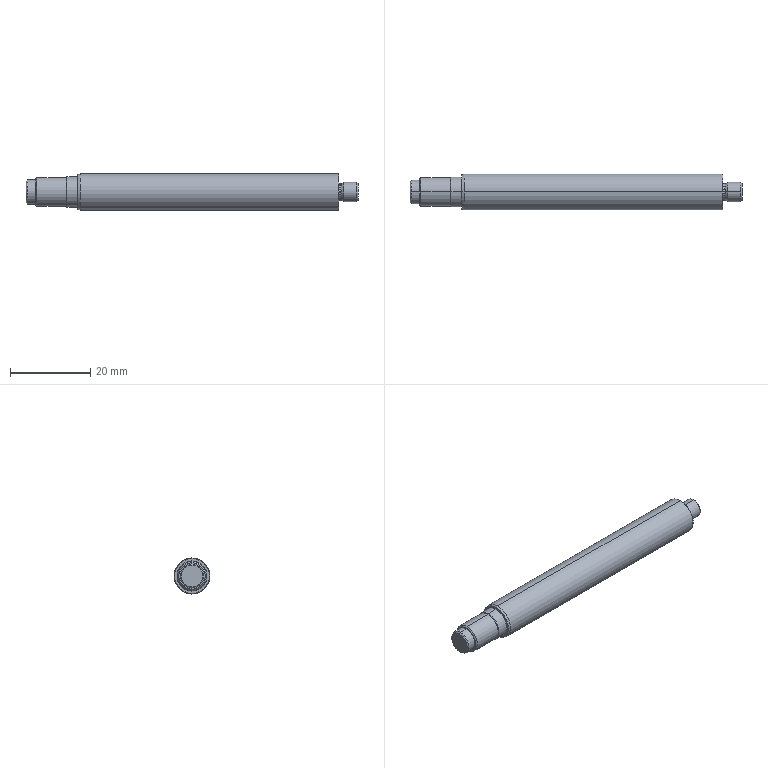Part | STEP file | 2026.6.15-Main Assembly图.sldasm-Part-245 | 1 solid | 35 faces | box 82.8 x 9 x 9 mm | volume 4725 mm3 | cone 12 | cylinder 12 | torus 6 | plane 5 | commonest cylinder face diameters 4.11 x2 4.8 x2 6 x2 7.2 x2 7.5 x2 9 x2
STEP:
#1=CARTESIAN_POINT('',(-1606.188,1424.264,3405.386));
#2=VERTEX_POINT('',#1);
#3=CARTESIAN_POINT('',(-1606.188,1424.264,3410.786));
#4=VERTEX_POINT('',#3);
#5=CARTESIAN_POINT('',(-1606.188,1424.264,3408.086));
#6=DIRECTION('',(1.,0.,0.));
#7=DIRECTION('',(0.,0.,-1.));
#8=AXIS2_PLACEMENT_3D('',#5,#6,#7);
#9=CIRCLE('',#8,2.7);
#10=EDGE_CURVE('',#2,#4,#9,.T.);
#11=ORIENTED_EDGE('',*,*,#10,.F.);
#12=CARTESIAN_POINT('',(-1606.188,1424.264,3408.086));
#13=DIRECTION('',(1.,0.,0.));
#14=DIRECTION('',(0.,0.,-1.));
#15=AXIS2_PLACEMENT_3D('',#12,#13,#14);
#16=CIRCLE('',#15,2.7);
#17=EDGE_CURVE('',#4,#2,#16,.T.);
#18=ORIENTED_EDGE('',*,*,#17,.F.);
#19=EDGE_LOOP('',(#11,#18));
#20=FACE_OUTER_BOUND('',#19,.T.);
#21=CARTESIAN_POINT('',(-1606.188,1424.264,3408.086));
#22=DIRECTION('',(-1.,0.,0.));
#23=DIRECTION('',(0.,0.,1.));
#24=AXIS2_PLACEMENT_3D('',#21,#22,#23);
#25=PLANE('',#24);
#26=ADVANCED_FACE('',(#20),#25,.T.);
#27=CARTESIAN_POINT('',(-1605.888,1424.264,3411.086));
#28=VERTEX_POINT('',#27);
#29=CARTESIAN_POINT('',(-1605.888,1424.264,3411.086));
#30=DIRECTION('',(0.7071,0.,0.7071));
#31=VECTOR('',#30,1000.);
#32=LINE('',#29,#31);
#33=EDGE_CURVE('',#4,#28,#32,.T.);
#34=ORIENTED_EDGE('',*,*,#33,.F.);
#35=ORIENTED_EDGE('',*,*,#17,.T.);
#36=CARTESIAN_POINT('',(-1605.888,1424.264,3405.086));
#37=VERTEX_POINT('',#36);
#38=CARTESIAN_POINT('',(-1605.888,1424.264,3405.086));
#39=DIRECTION('',(0.7071,0.,-0.7071));
#40=VECTOR('',#39,1000.);
#41=LINE('',#38,#40);
#42=EDGE_CURVE('',#2,#37,#41,.T.);
#43=ORIENTED_EDGE('',*,*,#42,.T.);
#44=CARTESIAN_POINT('',(-1605.888,1424.264,3408.086));
#45=DIRECTION('',(1.,0.,0.));
#46=DIRECTION('',(0.,0.,-1.));
#47=AXIS2_PLACEMENT_3D('',#44,#45,#46);
#48=CIRCLE('',#47,3.);
#49=EDGE_CURVE('',#28,#37,#48,.T.);
#50=ORIENTED_EDGE('',*,*,#49,.F.);
#51=EDGE_LOOP('',(#34,#35,#43,#50));
#52=FACE_OUTER_BOUND('',#51,.T.);
#53=CARTESIAN_POINT('',(-1605.888,1424.264,3408.086));
#54=DIRECTION('',(1.,0.,0.));
#55=DIRECTION('',(0.,0.,1.));
#56=AXIS2_PLACEMENT_3D('',#53,#54,#55);
#57=CONICAL_SURFACE('',#56,3.,0.7854);
#58=ADVANCED_FACE('',(#52),#57,.T.);
#59=CARTESIAN_POINT('',(-1523.388,1424.264,3410.186));
#60=VERTEX_POINT('',#59);
#61=CARTESIAN_POINT('',(-1523.388,1424.264,3405.986));
#62=VERTEX_POINT('',#61);
#63=CARTESIAN_POINT('',(-1523.388,1424.264,3408.086));
#64=DIRECTION('',(-1.,0.,0.));
#65=DIRECTION('',(0.,0.,1.));
#66=AXIS2_PLACEMENT_3D('',#63,#64,#65);
#67=CIRCLE('',#66,2.1);
#68=EDGE_CURVE('',#60,#62,#67,.T.);
#69=ORIENTED_EDGE('',*,*,#68,.F.);
#70=CARTESIAN_POINT('',(-1523.388,1424.264,3408.086));
#71=DIRECTION('',(-1.,0.,0.));
#72=DIRECTION('',(0.,0.,1.));
#73=AXIS2_PLACEMENT_3D('',#70,#71,#72);
#74=CIRCLE('',#73,2.1);
#75=EDGE_CURVE('',#62,#60,#74,.T.);
#76=ORIENTED_EDGE('',*,*,#75,.F.);
#77=EDGE_LOOP('',(#69,#76));
#78=FACE_OUTER_BOUND('',#77,.T.);
#79=CARTESIAN_POINT('',(-1523.388,1424.264,3408.086));
#80=DIRECTION('',(-1.,0.,0.));
#81=DIRECTION('',(0.,0.,1.));
#82=AXIS2_PLACEMENT_3D('',#79,#80,#81);
#83=PLANE('',#82);
#84=ADVANCED_FACE('',(#78),#83,.F.);
#85=CARTESIAN_POINT('',(-1603.788,1424.264,3411.086));
#86=VERTEX_POINT('',#85);
#87=CARTESIAN_POINT('',(-1603.788,1424.264,3411.086));
#88=DIRECTION('',(1.,0.,0.));
#89=VECTOR('',#88,1000.);
#90=LINE('',#87,#89);
#91=EDGE_CURVE('',#28,#86,#90,.T.);
#92=ORIENTED_EDGE('',*,*,#91,.F.);
#93=ORIENTED_EDGE('',*,*,#49,.T.);
#94=CARTESIAN_POINT('',(-1603.788,1424.264,3405.086));
#95=VERTEX_POINT('',#94);
#96=CARTESIAN_POINT('',(-1603.788,1424.264,3405.086));
#97=DIRECTION('',(1.,0.,0.));
#98=VECTOR('',#97,1000.);
#99=LINE('',#96,#98);
#100=EDGE_CURVE('',#37,#95,#99,.T.);
#101=ORIENTED_EDGE('',*,*,#100,.T.);
#102=CARTESIAN_POINT('',(-1603.788,1424.264,3408.086));
#103=DIRECTION('',(1.,0.,0.));
#104=DIRECTION('',(0.,0.,-1.));
#105=AXIS2_PLACEMENT_3D('',#102,#103,#104);
#106=CIRCLE('',#105,3.);
#107=EDGE_CURVE('',#86,#95,#106,.T.);
#108=ORIENTED_EDGE('',*,*,#107,.F.);
#109=EDGE_LOOP('',(#92,#93,#101,#108));
#110=FACE_OUTER_BOUND('',#109,.T.);
#111=CARTESIAN_POINT('',(-1603.788,1424.264,3408.086));
#112=DIRECTION('',(1.,0.,0.));
#113=DIRECTION('',(0.,0.,1.));
#114=AXIS2_PLACEMENT_3D('',#111,#112,#113);
#115=CYLINDRICAL_SURFACE('',#114,3.);
#116=ADVANCED_FACE('',(#110),#115,.T.);
#117=CARTESIAN_POINT('',(-1523.688,1424.264,3405.686));
#118=VERTEX_POINT('',#117);
#119=CARTESIAN_POINT('',(-1523.688,1424.264,3405.686));
#120=DIRECTION('',(0.7071,0.,0.7071));
#121=VECTOR('',#120,1000.);
#122=LINE('',#119,#121);
#123=EDGE_CURVE('',#118,#62,#122,.T.);
#124=ORIENTED_EDGE('',*,*,#123,.T.);
#125=ORIENTED_EDGE('',*,*,#75,.T.);
#126=CARTESIAN_POINT('',(-1523.688,1424.264,3410.486));
#127=VERTEX_POINT('',#126);
#128=CARTESIAN_POINT('',(-1523.688,1424.264,3410.486));
#129=DIRECTION('',(0.7071,0.,-0.7071));
#130=VECTOR('',#129,1000.);
#131=LINE('',#128,#130);
#132=EDGE_CURVE('',#127,#60,#131,.T.);
#133=ORIENTED_EDGE('',*,*,#132,.F.);
#134=CARTESIAN_POINT('',(-1523.688,1424.264,3408.086));
#135=DIRECTION('',(-1.,0.,0.));
#136=DIRECTION('',(0.,0.,1.));
#137=AXIS2_PLACEMENT_3D('',#134,#135,#136);
#138=CIRCLE('',#137,2.4);
#139=EDGE_CURVE('',#118,#127,#138,.T.);
#140=ORIENTED_EDGE('',*,*,#139,.F.);
#141=EDGE_LOOP('',(#124,#125,#133,#140));
#142=FACE_OUTER_BOUND('',#141,.T.);
#143=CARTESIAN_POINT('',(-1523.688,1424.264,3408.086));
#144=DIRECTION('',(-1.,0.,0.));
#145=DIRECTION('',(0.,0.,-1.));
#146=AXIS2_PLACEMENT_3D('',#143,#144,#145);
#147=CONICAL_SURFACE('',#146,2.4,0.7854);
#148=ADVANCED_FACE('',(#142),#147,.T.);
#149=CARTESIAN_POINT('',(-1603.788,1424.264,3404.786));
#150=VERTEX_POINT('',#149);
#151=CARTESIAN_POINT('',(-1603.788,1424.264,3411.386));
#152=VERTEX_POINT('',#151);
#153=CARTESIAN_POINT('',(-1603.788,1424.264,3408.086));
#154=DIRECTION('',(1.,0.,0.));
#155=DIRECTION('',(0.,0.,-1.));
#156=AXIS2_PLACEMENT_3D('',#153,#154,#155);
#157=CIRCLE('',#156,3.3);
#158=EDGE_CURVE('',#150,#152,#157,.T.);
#159=ORIENTED_EDGE('',*,*,#158,.F.);
#160=CARTESIAN_POINT('',(-1603.788,1424.264,3408.086));
#161=DIRECTION('',(1.,0.,0.));
#162=DIRECTION('',(0.,0.,-1.));
#163=AXIS2_PLACEMENT_3D('',#160,#161,#162);
#164=CIRCLE('',#163,3.3);
#165=EDGE_CURVE('',#152,#150,#164,.T.);
#166=ORIENTED_EDGE('',*,*,#165,.F.);
#167=EDGE_LOOP('',(#159,#166));
#168=FACE_OUTER_BOUND('',#167,.T.);
#169=CARTESIAN_POINT('',(-1603.788,1424.264,3408.086));
#170=DIRECTION('',(1.,0.,0.));
#171=DIRECTION('',(0.,0.,-1.));
#172=AXIS2_PLACEMENT_3D('',#169,#170,#171);
#173=CIRCLE('',#172,3.);
#174=EDGE_CURVE('',#95,#86,#173,.T.);
#175=ORIENTED_EDGE('',*,*,#174,.T.);
#176=ORIENTED_EDGE('',*,*,#107,.T.);
#177=EDGE_LOOP('',(#175,#176));
#178=FACE_BOUND('',#177,.T.);
#179=CARTESIAN_POINT('',(-1603.788,1425.764,3408.086));
#180=DIRECTION('',(-1.,0.,0.));
#181=DIRECTION('',(0.,0.,1.));
#182=AXIS2_PLACEMENT_3D('',#179,#180,#181);
#183=PLANE('',#182);
#184=ADVANCED_FACE('',(#168,#178),#183,.T.);
#185=CARTESIAN_POINT('',(-1526.988,1424.264,3405.686));
#186=VERTEX_POINT('',#185);
#187=CARTESIAN_POINT('',(-1528.188,1424.264,3405.686));
#188=DIRECTION('',(1.,0.,0.));
#189=VECTOR('',#188,1000.);
#190=LINE('',#187,#189);
#191=EDGE_CURVE('',#186,#118,#190,.T.);
#192=ORIENTED_EDGE('',*,*,#191,.T.);
#193=ORIENTED_EDGE('',*,*,#139,.T.);
#194=CARTESIAN_POINT('',(-1526.988,1424.264,3410.486));
#195=VERTEX_POINT('',#194);
#196=CARTESIAN_POINT('',(-1528.188,1424.264,3410.486));
#197=DIRECTION('',(1.,0.,0.));
#198=VECTOR('',#197,1000.);
#199=LINE('',#196,#198);
#200=EDGE_CURVE('',#195,#127,#199,.T.);
#201=ORIENTED_EDGE('',*,*,#200,.F.);
#202=CARTESIAN_POINT('',(-1526.988,1424.264,3408.086));
#203=DIRECTION('',(-1.,0.,0.));
#204=DIRECTION('',(0.,0.,-1.));
#205=AXIS2_PLACEMENT_3D('',#202,#203,#204);
#206=CIRCLE('',#205,2.4);
#207=EDGE_CURVE('',#186,#195,#206,.T.);
#208=ORIENTED_EDGE('',*,*,#207,.F.);
#209=EDGE_LOOP('',(#192,#193,#201,#208));
#210=FACE_OUTER_BOUND('',#209,.T.);
#211=CARTESIAN_POINT('',(-1528.188,1424.264,3408.086));
#212=DIRECTION('',(-1.,0.,0.));
#213=DIRECTION('',(0.,0.,-1.));
#214=AXIS2_PLACEMENT_3D('',#211,#212,#213);
#215=CYLINDRICAL_SURFACE('',#214,2.4);
#216=ADVANCED_FACE('',(#210),#215,.T.);
#217=CARTESIAN_POINT('',(-1603.488,1424.264,3411.686));
#218=VERTEX_POINT('',#217);
#219=CARTESIAN_POINT('',(-1603.488,1424.264,3411.686));
#220=DIRECTION('',(0.7071,0.,0.7071));
#221=VECTOR('',#220,1000.);
#222=LINE('',#219,#221);
#223=EDGE_CURVE('',#152,#218,#222,.T.);
#224=ORIENTED_EDGE('',*,*,#223,.F.);
#225=ORIENTED_EDGE('',*,*,#165,.T.);
#226=CARTESIAN_POINT('',(-1603.488,1424.264,3404.486));
#227=VERTEX_POINT('',#226);
#228=CARTESIAN_POINT('',(-1603.488,1424.264,3404.486));
#229=DIRECTION('',(0.7071,0.,-0.7071));
#230=VECTOR('',#229,1000.);
#231=LINE('',#228,#230);
#232=EDGE_CURVE('',#150,#227,#231,.T.);
#233=ORIENTED_EDGE('',*,*,#232,.T.);
#234=CARTESIAN_POINT('',(-1603.488,1424.264,3408.086));
#235=DIRECTION('',(1.,0.,0.));
#236=DIRECTION('',(0.,0.,-1.));
#237=AXIS2_PLACEMENT_3D('',#234,#235,#236);
#238=CIRCLE('',#237,3.6);
#239=EDGE_CURVE('',#218,#227,#238,.T.);
#240=ORIENTED_EDGE('',*,*,#239,.F.);
#241=EDGE_LOOP('',(#224,#225,#233,#240));
#242=FACE_OUTER_BOUND('',#241,.T.);
#243=CARTESIAN_POINT('',(-1603.488,1424.264,3408.086));
#244=DIRECTION('',(1.,0.,0.));
#245=DIRECTION('',(0.,0.,1.));
#246=AXIS2_PLACEMENT_3D('',#243,#244,#245);
#247=CONICAL_SURFACE('',#246,3.6,0.7854);
#248=ADVANCED_FACE('',(#242),#247,.T.);
#249=CARTESIAN_POINT('',(-1527.53,1424.264,3410.173));
#250=VERTEX_POINT('',#249);
#251=CARTESIAN_POINT('',(-1526.988,1424.264,3410.486));
#252=DIRECTION('',(0.866,0.,0.5));
#253=VECTOR('',#252,1000.);
#254=LINE('',#251,#253);
#255=EDGE_CURVE('',#250,#195,#254,.T.);
#256=ORIENTED_EDGE('',*,*,#255,.F.);
#257=CARTESIAN_POINT('',(-1527.53,1424.264,3405.999));
#258=VERTEX_POINT('',#257);
#259=CARTESIAN_POINT('',(-1527.53,1424.264,3408.086));
#260=DIRECTION('',(1.,0.,0.));
#261=DIRECTION('',(0.,0.,1.));
#262=AXIS2_PLACEMENT_3D('',#259,#260,#261);
#263=CIRCLE('',#262,2.087);
#264=EDGE_CURVE('',#250,#258,#263,.T.);
#265=ORIENTED_EDGE('',*,*,#264,.T.);
#266=CARTESIAN_POINT('',(-1526.988,1424.264,3405.686));
#267=DIRECTION('',(0.866,0.,-0.5));
#268=VECTOR('',#267,1000.);
#269=LINE('',#266,#268);
#270=EDGE_CURVE('',#258,#186,#269,.T.);
#271=ORIENTED_EDGE('',*,*,#270,.T.);
#272=ORIENTED_EDGE('',*,*,#207,.T.);
#273=EDGE_LOOP('',(#256,#265,#271,#272));
#274=FACE_OUTER_BOUND('',#273,.T.);
#275=CARTESIAN_POINT('',(-1526.988,1424.264,3408.086));
#276=DIRECTION('',(1.,0.,0.));
#277=DIRECTION('',(0.,0.,1.));
#278=AXIS2_PLACEMENT_3D('',#275,#276,#277);
#279=CONICAL_SURFACE('',#278,2.4,0.5236);
#280=ADVANCED_FACE('',(#274),#279,.T.);
#281=CARTESIAN_POINT('',(-1596.138,1424.264,3411.686));
#282=VERTEX_POINT('',#281);
#283=CARTESIAN_POINT('',(-1595.988,1424.264,3411.686));
#284=DIRECTION('',(1.,0.,0.));
#285=VECTOR('',#284,1000.);
#286=LINE('',#283,#285);
#287=EDGE_CURVE('',#218,#282,#286,.T.);
#288=ORIENTED_EDGE('',*,*,#287,.F.);
#289=ORIENTED_EDGE('',*,*,#239,.T.);
#290=CARTESIAN_POINT('',(-1596.138,1424.264,3404.486));
#291=VERTEX_POINT('',#290);
#292=CARTESIAN_POINT('',(-1595.988,1424.264,3404.486));
#293=DIRECTION('',(1.,0.,0.));
#294=VECTOR('',#293,1000.);
#295=LINE('',#292,#294);
#296=EDGE_CURVE('',#227,#291,#295,.T.);
#297=ORIENTED_EDGE('',*,*,#296,.T.);
#298=CARTESIAN_POINT('',(-1596.138,1424.264,3408.086));
#299=DIRECTION('',(1.,0.,0.));
#300=DIRECTION('',(0.,0.,-1.));
#301=AXIS2_PLACEMENT_3D('',#298,#299,#300);
#302=CIRCLE('',#301,3.6);
#303=EDGE_CURVE('',#282,#291,#302,.T.);
#304=ORIENTED_EDGE('',*,*,#303,.F.);
#305=EDGE_LOOP('',(#288,#289,#297,#304));
#306=FACE_OUTER_BOUND('',#305,.T.);
#307=CARTESIAN_POINT('',(-1595.988,1424.264,3408.086));
#308=DIRECTION('',(1.,0.,0.));
#309=DIRECTION('',(0.,0.,1.));
#310=AXIS2_PLACEMENT_3D('',#307,#308,#309);
#311=CYLINDRICAL_SURFACE('',#310,3.6);
#312=ADVANCED_FACE('',(#306),#311,.T.);
#313=CARTESIAN_POINT('',(-1527.65,1424.264,3406.031));
#314=VERTEX_POINT('',#313);
#315=CARTESIAN_POINT('',(-1527.65,1424.264,3405.791));
#316=DIRECTION('',(0.,-1.,0.));
#317=DIRECTION('',(0.9969,0.,-0.0785));
#318=AXIS2_PLACEMENT_3D('',#315,#316,#317);
#319=CIRCLE('',#318,0.24);
#320=EDGE_CURVE('',#258,#314,#319,.T.);
#321=ORIENTED_EDGE('',*,*,#320,.T.);
#322=CARTESIAN_POINT('',(-1527.65,1424.264,3410.141));
#323=VERTEX_POINT('',#322);
#324=CARTESIAN_POINT('',(-1527.65,1424.264,3408.086));
#325=DIRECTION('',(-1.,0.,0.));
#326=DIRECTION('',(0.,0.,-1.));
#327=AXIS2_PLACEMENT_3D('',#324,#325,#326);
#328=CIRCLE('',#327,2.055);
#329=EDGE_CURVE('',#323,#314,#328,.T.);
#330=ORIENTED_EDGE('',*,*,#329,.F.);
#331=CARTESIAN_POINT('',(-1527.65,1424.264,3410.381));
#332=DIRECTION('',(0.,1.,0.));
#333=DIRECTION('',(-0.9969,0.,0.0785));
#334=AXIS2_PLACEMENT_3D('',#331,#332,#333);
#335=CIRCLE('',#334,0.24);
#336=EDGE_CURVE('',#250,#323,#335,.T.);
#337=ORIENTED_EDGE('',*,*,#336,.F.);
#338=CARTESIAN_POINT('',(-1527.53,1424.264,3408.086));
#339=DIRECTION('',(1.,0.,0.));
#340=DIRECTION('',(0.,0.,1.));
#341=AXIS2_PLACEMENT_3D('',#338,#339,#340);
#342=CIRCLE('',#341,2.087);
#343=EDGE_CURVE('',#258,#250,#342,.T.);
#344=ORIENTED_EDGE('',*,*,#343,.F.);
#345=EDGE_LOOP('',(#321,#330,#337,#344));
#346=FACE_OUTER_BOUND('',#345,.T.);
#347=CARTESIAN_POINT('',(-1527.65,1424.264,3408.086));
#348=DIRECTION('',(-1.,0.,0.));
#349=DIRECTION('',(0.,0.,-1.));
#350=AXIS2_PLACEMENT_3D('',#347,#348,#349);
#351=TOROIDAL_SURFACE('',#350,2.295,0.24);
#352=ADVANCED_FACE('',(#346),#351,.F.);
#353=CARTESIAN_POINT('',(-1595.988,1424.264,3411.836));
#354=VERTEX_POINT('',#353);
#355=CARTESIAN_POINT('',(-1595.988,1424.264,3411.836));
#356=DIRECTION('',(0.7071,0.,0.7071));
#357=VECTOR('',#356,1000.);
#358=LINE('',#355,#357);
#359=EDGE_CURVE('',#282,#354,#358,.T.);
#360=ORIENTED_EDGE('',*,*,#359,.F.);
#361=ORIENTED_EDGE('',*,*,#303,.T.);
#362=CARTESIAN_POINT('',(-1595.988,1424.264,3404.336));
#363=VERTEX_POINT('',#362);
#364=CARTESIAN_POINT('',(-1595.988,1424.264,3404.336));
#365=DIRECTION('',(0.7071,0.,-0.7071));
#366=VECTOR('',#365,1000.);
#367=LINE('',#364,#366);
#368=EDGE_CURVE('',#291,#363,#367,.T.);
#369=ORIENTED_EDGE('',*,*,#368,.T.);
#370=CARTESIAN_POINT('',(-1595.988,1424.264,3408.086));
#371=DIRECTION('',(1.,0.,0.));
#372=DIRECTION('',(0.,0.,-1.));
#373=AXIS2_PLACEMENT_3D('',#370,#371,#372);
#374=CIRCLE('',#373,3.75);
#375=EDGE_CURVE('',#354,#363,#374,.T.);
#376=ORIENTED_EDGE('',*,*,#375,.F.);
#377=EDGE_LOOP('',(#360,#361,#369,#376));
#378=FACE_OUTER_BOUND('',#377,.T.);
#379=CARTESIAN_POINT('',(-1595.988,1424.264,3408.086));
#380=DIRECTION('',(1.,0.,0.));
#381=DIRECTION('',(0.,0.,1.));
#382=AXIS2_PLACEMENT_3D('',#379,#380,#381);
#383=CONICAL_SURFACE('',#382,3.75,0.7854);
#384=ADVANCED_FACE('',(#378),#383,.T.);
#385=CARTESIAN_POINT('',(-1527.948,1424.264,3410.141));
#386=VERTEX_POINT('',#385);
#387=CARTESIAN_POINT('',(-1624.188,1424.264,3410.141));
#388=DIRECTION('',(1.,0.,0.));
#389=VECTOR('',#388,1000.);
#390=LINE('',#387,#389);
#391=EDGE_CURVE('',#386,#323,#390,.T.);
#392=ORIENTED_EDGE('',*,*,#391,.F.);
#393=CARTESIAN_POINT('',(-1527.948,1424.264,3406.031));
#394=VERTEX_POINT('',#393);
#395=CARTESIAN_POINT('',(-1527.948,1424.264,3408.086));
#396=DIRECTION('',(1.,0.,0.));
#397=DIRECTION('',(0.,-1.,0.));
#398=AXIS2_PLACEMENT_3D('',#395,#396,#397);
#399=CIRCLE('',#398,2.055);
#400=EDGE_CURVE('',#386,#394,#399,.T.);
#401=ORIENTED_EDGE('',*,*,#400,.T.);
#402=CARTESIAN_POINT('',(-1624.188,1424.264,3406.031));
#403=DIRECTION('',(1.,0.,0.));
#404=VECTOR('',#403,1000.);
#405=LINE('',#402,#404);
#406=EDGE_CURVE('',#394,#314,#405,.T.);
#407=ORIENTED_EDGE('',*,*,#406,.T.);
#408=CARTESIAN_POINT('',(-1527.65,1424.264,3408.086));
#409=DIRECTION('',(-1.,0.,0.));
#410=DIRECTION('',(0.,0.,-1.));
#411=AXIS2_PLACEMENT_3D('',#408,#409,#410);
#412=CIRCLE('',#411,2.055);
#413=EDGE_CURVE('',#314,#323,#412,.T.);
#414=ORIENTED_EDGE('',*,*,#413,.T.);
#415=EDGE_LOOP('',(#392,#401,#407,#414));
#416=FACE_OUTER_BOUND('',#415,.T.);
#417=CARTESIAN_POINT('',(-1624.188,1424.264,3408.086));
#418=DIRECTION('',(1.,0.,0.));
#419=DIRECTION('',(0.,0.,1.));
#420=AXIS2_PLACEMENT_3D('',#417,#418,#419);
#421=CYLINDRICAL_SURFACE('',#420,2.055);
#422=ADVANCED_FACE('',(#416),#421,.T.);
#423=CARTESIAN_POINT('',(-1593.288,1424.264,3411.836));
#424=VERTEX_POINT('',#423);
#425=CARTESIAN_POINT('',(-1593.288,1424.264,3411.836));
#426=DIRECTION('',(1.,0.,0.));
#427=VECTOR('',#426,1000.);
#428=LINE('',#425,#427);
#429=EDGE_CURVE('',#354,#424,#428,.T.);
#430=ORIENTED_EDGE('',*,*,#429,.F.);
#431=ORIENTED_EDGE('',*,*,#375,.T.);
#432=CARTESIAN_POINT('',(-1593.288,1424.264,3404.336));
#433=VERTEX_POINT('',#432);
#434=CARTESIAN_POINT('',(-1593.288,1424.264,3404.336));
#435=DIRECTION('',(1.,0.,0.));
#436=VECTOR('',#435,1000.);
#437=LINE('',#434,#436);
#438=EDGE_CURVE('',#363,#433,#437,.T.);
#439=ORIENTED_EDGE('',*,*,#438,.T.);
#440=CARTESIAN_POINT('',(-1593.288,1424.264,3408.086));
#441=DIRECTION('',(1.,0.,0.));
#442=DIRECTION('',(0.,0.,-1.));
#443=AXIS2_PLACEMENT_3D('',#440,#441,#442);
#444=CIRCLE('',#443,3.75);
#445=EDGE_CURVE('',#424,#433,#444,.T.);
#446=ORIENTED_EDGE('',*,*,#445,.F.);
#447=EDGE_LOOP('',(#430,#431,#439,#446));
#448=FACE_OUTER_BOUND('',#447,.T.);
#449=CARTESIAN_POINT('',(-1593.288,1424.264,3408.086));
#450=DIRECTION('',(1.,0.,0.));
#451=DIRECTION('',(0.,0.,1.));
#452=AXIS2_PLACEMENT_3D('',#449,#450,#451);
#453=CYLINDRICAL_SURFACE('',#452,3.75);
#454=ADVANCED_FACE('',(#448),#453,.T.);
#455=CARTESIAN_POINT('',(-1528.188,1424.264,3410.381));
#456=VERTEX_POINT('',#455);
#457=CARTESIAN_POINT('',(-1527.948,1424.264,3410.381));
#458=DIRECTION('',(0.,1.,0.));
#459=DIRECTION('',(0.9969,0.,-0.0785));
#460=AXIS2_PLACEMENT_3D('',#457,#458,#459);
#461=CIRCLE('',#460,0.24);
#462=EDGE_CURVE('',#386,#456,#461,.T.);
#463=ORIENTED_EDGE('',*,*,#462,.F.);
#464=CARTESIAN_POINT('',(-1527.948,1424.264,3408.086));
#465=DIRECTION('',(1.,0.,0.));
#466=DIRECTION('',(0.,-1.,0.));
#467=AXIS2_PLACEMENT_3D('',#464,#465,#466);
#468=CIRCLE('',#467,2.055);
#469=EDGE_CURVE('',#394,#386,#468,.T.);
#470=ORIENTED_EDGE('',*,*,#469,.F.);
#471=CARTESIAN_POINT('',(-1528.188,1424.264,3405.791));
#472=VERTEX_POINT('',#471);
#473=CARTESIAN_POINT('',(-1527.948,1424.264,3405.791));
#474=DIRECTION('',(0.,-1.,0.));
#475=DIRECTION('',(-0.9969,0.,0.0785));
#476=AXIS2_PLACEMENT_3D('',#473,#474,#475);
#477=CIRCLE('',#476,0.24);
#478=EDGE_CURVE('',#394,#472,#477,.T.);
#479=ORIENTED_EDGE('',*,*,#478,.T.);
#480=CARTESIAN_POINT('',(-1528.188,1424.264,3408.086));
#481=DIRECTION('',(-1.,0.,0.));
#482=DIRECTION('',(0.,0.,-1.));
#483=AXIS2_PLACEMENT_3D('',#480,#481,#482);
#484=CIRCLE('',#483,2.295);
#485=EDGE_CURVE('',#456,#472,#484,.T.);
#486=ORIENTED_EDGE('',*,*,#485,.F.);
#487=EDGE_LOOP('',(#463,#470,#479,#486));
#488=FACE_OUTER_BOUND('',#487,.T.);
#489=CARTESIAN_POINT('',(-1527.948,1424.264,3408.086));
#490=DIRECTION('',(1.,0.,0.));
#491=DIRECTION('',(0.,0.,1.));
#492=AXIS2_PLACEMENT_3D('',#489,#490,#491);
#493=TOROIDAL_SURFACE('',#492,2.295,0.24);
#494=ADVANCED_FACE('',(#488),#493,.F.);
#495=CARTESIAN_POINT('',(-1593.288,1424.264,3403.747));
#496=VERTEX_POINT('',#495);
#497=CARTESIAN_POINT('',(-1593.288,1424.264,3412.426));
#498=VERTEX_POINT('',#497);
#499=CARTESIAN_POINT('',(-1593.288,1424.264,3408.086));
#500=DIRECTION('',(1.,0.,0.));
#501=DIRECTION('',(0.,0.,-1.));
#502=AXIS2_PLACEMENT_3D('',#499,#500,#501);
#503=CIRCLE('',#502,4.339);
#504=EDGE_CURVE('',#496,#498,#503,.T.);
#505=ORIENTED_EDGE('',*,*,#504,.F.);
#506=CARTESIAN_POINT('',(-1593.288,1424.264,3408.086));
#507=DIRECTION('',(1.,0.,0.));
#508=DIRECTION('',(0.,0.,-1.));
#509=AXIS2_PLACEMENT_3D('',#506,#507,#508);
#510=CIRCLE('',#509,4.339);
#511=EDGE_CURVE('',#498,#496,#510,.T.);
#512=ORIENTED_EDGE('',*,*,#511,.F.);
#513=EDGE_LOOP('',(#505,#512));
#514=FACE_OUTER_BOUND('',#513,.T.);
#515=CARTESIAN_POINT('',(-1593.288,1424.264,3408.086));
#516=DIRECTION('',(1.,0.,0.));
#517=DIRECTION('',(0.,0.,-1.));
#518=AXIS2_PLACEMENT_3D('',#515,#516,#517);
#519=CIRCLE('',#518,3.75);
#520=EDGE_CURVE('',#433,#424,#519,.T.);
#521=ORIENTED_EDGE('',*,*,#520,.T.);
#522=ORIENTED_EDGE('',*,*,#445,.T.);
#523=EDGE_LOOP('',(#521,#522));
#524=FACE_BOUND('',#523,.T.);
#525=CARTESIAN_POINT('',(-1593.288,1426.139,3408.086));
#526=DIRECTION('',(-1.,0.,0.));
#527=DIRECTION('',(0.,0.,1.));
#528=AXIS2_PLACEMENT_3D('',#525,#526,#527);
#529=PLANE('',#528);
#530=ADVANCED_FACE('',(#514,#524),#529,.T.);
#531=CARTESIAN_POINT('',(-1528.188,1419.914,3408.086));
#532=VERTEX_POINT('',#531);
#533=CARTESIAN_POINT('',(-1528.188,1424.264,3412.436));
#534=VERTEX_POINT('',#533);
#535=CARTESIAN_POINT('',(-1528.188,1424.264,3408.086));
#536=DIRECTION('',(-1.,0.,0.));
#537=DIRECTION('',(0.,0.,-1.));
#538=AXIS2_PLACEMENT_3D('',#535,#536,#537);
#539=CIRCLE('',#538,4.35);
#540=EDGE_CURVE('',#532,#534,#539,.T.);
#541=ORIENTED_EDGE('',*,*,#540,.F.);
#542=CARTESIAN_POINT('',(-1528.188,1424.264,3403.736));
#543=VERTEX_POINT('',#542);
#544=CARTESIAN_POINT('',(-1528.188,1424.264,3403.736));
#545=CARTESIAN_POINT('',(-1528.188,1424.253,3403.736));
#546=CARTESIAN_POINT('',(-1528.188,1424.225,3403.736));
#547=CARTESIAN_POINT('',(-1528.188,1424.157,3403.738));
#548=CARTESIAN_POINT('',(-1528.188,1424.13,3403.738));
#549=CARTESIAN_POINT('',(-1528.188,1424.084,3403.74));
#550=CARTESIAN_POINT('',(-1528.188,1424.067,3403.741));
#551=CARTESIAN_POINT('',(-1528.188,1424.041,3403.742));
#552=CARTESIAN_POINT('',(-1528.188,1424.027,3403.743));
#553=CARTESIAN_POINT('',(-1528.188,1424.01,3403.744));
#554=CARTESIAN_POINT('',(-1528.188,1424.002,3403.744));
#555=CARTESIAN_POINT('',(-1528.188,1423.998,3403.744));
#556=CARTESIAN_POINT('',(-1528.188,1423.996,3403.745));
#557=CARTESIAN_POINT('',(-1528.188,1423.994,3403.745));
#558=CARTESIAN_POINT('',(-1528.188,1423.94,3403.748));
#559=CARTESIAN_POINT('',(-1528.188,1423.891,3403.752));
#560=CARTESIAN_POINT('',(-1528.188,1423.824,3403.759));
#561=CARTESIAN_POINT('',(-1528.188,1423.802,3403.761));
#562=CARTESIAN_POINT('',(-1528.188,1423.772,3403.764));
#563=CARTESIAN_POINT('',(-1528.188,1423.757,3403.766));
#564=CARTESIAN_POINT('',(-1528.188,1423.741,3403.768));
#565=CARTESIAN_POINT('',(-1528.188,1423.734,3403.769));
#566=CARTESIAN_POINT('',(-1528.188,1423.729,3403.769));
#567=CARTESIAN_POINT('',(-1528.188,1423.727,3403.769));
#568=CARTESIAN_POINT('',(-1528.188,1423.635,3403.781));
#569=CARTESIAN_POINT('',(-1528.188,1423.546,3403.795));
#570=CARTESIAN_POINT('',(-1528.188,1423.413,3403.82));
#571=CARTESIAN_POINT('',(-1528.188,1423.347,3403.834));
#572=CARTESIAN_POINT('',(-1528.188,1423.27,3403.851));
#573=CARTESIAN_POINT('',(-1528.188,1423.232,3403.861));
#574=CARTESIAN_POINT('',(-1528.188,1423.213,3403.865));
#575=CARTESIAN_POINT('',(-1528.188,1423.203,3403.868));
#576=CARTESIAN_POINT('',(-1528.188,1423.198,3403.869));
#577=CARTESIAN_POINT('',(-1528.188,1423.196,3403.869));
#578=CARTESIAN_POINT('',(-1528.188,1423.195,3403.87));
#579=CARTESIAN_POINT('',(-1528.188,1423.194,3403.87));
#580=CARTESIAN_POINT('',(-1528.188,1423.183,3403.873));
#581=CARTESIAN_POINT('',(-1528.188,1423.157,3403.879));
#582=CARTESIAN_POINT('',(-1528.188,1423.093,3403.897));
#583=CARTESIAN_POINT('',(-1528.188,1423.068,3403.904));
#584=CARTESIAN_POINT('',(-1528.188,1423.025,3403.917));
#585=CARTESIAN_POINT('',(-1528.188,1423.009,3403.921));
#586=CARTESIAN_POINT('',(-1528.188,1422.985,3403.929));
#587=CARTESIAN_POINT('',(-1528.188,1422.972,3403.933));
#588=CARTESIAN_POINT('',(-1528.188,1422.957,3403.937));
#589=CARTESIAN_POINT('',(-1528.188,1422.949,3403.94));
#590=CARTESIAN_POINT('',(-1528.188,1422.945,3403.941));
#591=CARTESIAN_POINT('',(-1528.188,1422.943,3403.942));
#592=CARTESIAN_POINT('',(-1528.188,1422.942,3403.942));
#593=CARTESIAN_POINT('',(-1528.188,1422.891,3403.958));
#594=CARTESIAN_POINT('',(-1528.188,1422.846,3403.974));
#595=CARTESIAN_POINT('',(-1528.188,1422.784,3403.996));
#596=CARTESIAN_POINT('',(-1528.188,1422.765,3404.003));
#597=CARTESIAN_POINT('',(-1528.188,1422.737,3404.013));
#598=CARTESIAN_POINT('',(-1528.188,1422.724,3404.018));
#599=CARTESIAN_POINT('',(-1528.188,1422.709,3404.024));
#600=CARTESIAN_POINT('',(-1528.188,1422.702,3404.026));
#601=CARTESIAN_POINT('',(-1528.188,1422.698,3404.028));
#602=CARTESIAN_POINT('',(-1528.188,1422.696,3404.029));
#603=CARTESIAN_POINT('',(-1528.188,1422.612,3404.061));
#604=CARTESIAN_POINT('',(-1528.188,1422.532,3404.095));
#605=CARTESIAN_POINT('',(-1528.188,1422.413,3404.15));
#606=CARTESIAN_POINT('',(-1528.188,1422.353,3404.178));
#607=CARTESIAN_POINT('',(-1528.188,1422.285,3404.213));
#608=CARTESIAN_POINT('',(-1528.188,1422.256,3404.228));
#609=CARTESIAN_POINT('',(-1528.188,1422.237,3404.238));
#610=CARTESIAN_POINT('',(-1528.188,1422.226,3404.243));
#611=CARTESIAN_POINT('',(-1528.188,1422.144,3404.287));
#612=CARTESIAN_POINT('',(-1528.188,1422.073,3404.328));
#613=CARTESIAN_POINT('',(-1528.188,1421.967,3404.392));
#614=CARTESIAN_POINT('',(-1528.188,1421.915,3404.425));
#615=CARTESIAN_POINT('',(-1528.188,1421.854,3404.465));
#616=CARTESIAN_POINT('',(-1528.188,1421.824,3404.485));
#617=CARTESIAN_POINT('',(-1528.188,1421.809,3404.495));
#618=CARTESIAN_POINT('',(-1528.188,1421.802,3404.5));
#619=CARTESIAN_POINT('',(-1528.188,1421.798,3404.503));
#620=CARTESIAN_POINT('',(-1528.188,1421.797,3404.504));
#621=CARTESIAN_POINT('',(-1528.188,1421.796,3404.505));
#622=CARTESIAN_POINT('',(-1528.188,1421.795,3404.505));
#623=CARTESIAN_POINT('',(-1528.188,1421.787,3404.511));
#624=CARTESIAN_POINT('',(-1528.188,1421.766,3404.525));
#625=CARTESIAN_POINT('',(-1528.188,1421.716,3404.561));
#626=CARTESIAN_POINT('',(-1528.188,1421.696,3404.575));
#627=CARTESIAN_POINT('',(-1528.188,1421.662,3404.601));
#628=CARTESIAN_POINT('',(-1528.188,1421.643,3404.615));
#629=CARTESIAN_POINT('',(-1528.188,1421.62,3404.632));
#630=CARTESIAN_POINT('',(-1528.188,1421.609,3404.64));
#631=CARTESIAN_POINT('',(-1528.188,1421.602,3404.646));
#632=CARTESIAN_POINT('',(-1528.188,1421.598,3404.649));
#633=CARTESIAN_POINT('',(-1528.188,1421.544,3404.691));
#634=CARTESIAN_POINT('',(-1528.188,1421.503,3404.725));
#635=CARTESIAN_POINT('',(-1528.188,1421.456,3404.764));
#636=CARTESIAN_POINT('',(-1528.188,1421.442,3404.776));
#637=CARTESIAN_POINT('',(-1528.188,1421.425,3404.79));
#638=CARTESIAN_POINT('',(-1528.188,1421.418,3404.797));
#639=CARTESIAN_POINT('',(-1528.188,1421.41,3404.803));
#640=CARTESIAN_POINT('',(-1528.188,1421.407,3404.806));
#641=CARTESIAN_POINT('',(-1528.188,1421.406,3404.807));
#642=CARTESIAN_POINT('',(-1528.188,1421.405,3404.808));
#643=CARTESIAN_POINT('',(-1528.188,1421.405,3404.808));
#644=CARTESIAN_POINT('',(-1528.188,1421.289,3404.909));
#645=CARTESIAN_POINT('',(-1528.188,1421.18,3405.015));
#646=CARTESIAN_POINT('',(-1528.188,1421.025,3405.182));
#647=CARTESIAN_POINT('',(-1528.188,1420.975,3405.239));
#648=CARTESIAN_POINT('',(-1528.188,1420.902,3405.327));
#649=CARTESIAN_POINT('',(-1528.188,1420.866,3405.371));
#650=CARTESIAN_POINT('',(-1528.188,1420.83,3405.416));
#651=CARTESIAN_POINT('',(-1528.188,1420.807,3405.446));
#652=CARTESIAN_POINT('',(-1528.188,1420.795,3405.462));
#653=CARTESIAN_POINT('',(-1528.188,1420.608,3405.712));
#654=CARTESIAN_POINT('',(-1528.188,1420.465,3405.952));
#655=CARTESIAN_POINT('',(-1528.188,1420.294,3406.304));
#656=CARTESIAN_POINT('',(-1528.188,1420.244,3406.42));
#657=CARTESIAN_POINT('',(-1528.188,1420.179,3406.591));
#658=CARTESIAN_POINT('',(-1528.188,1420.159,3406.647));
#659=CARTESIAN_POINT('',(-1528.188,1420.131,3406.731));
#660=CARTESIAN_POINT('',(-1528.188,1420.117,3406.772));
#661=CARTESIAN_POINT('',(-1528.188,1420.103,3406.821));
#662=CARTESIAN_POINT('',(-1528.188,1420.096,3406.841));
#663=CARTESIAN_POINT('',(-1528.188,1420.092,3406.855));
#664=CARTESIAN_POINT('',(-1528.188,1420.09,3406.862));
#665=CARTESIAN_POINT('',(-1528.188,1420.06,3406.967));
#666=CARTESIAN_POINT('',(-1528.188,1420.034,3407.067));
#667=CARTESIAN_POINT('',(-1528.188,1420.002,3407.218));
#668=CARTESIAN_POINT('',(-1528.188,1419.987,3407.293));
#669=CARTESIAN_POINT('',(-1528.188,1419.971,3407.382));
#670=CARTESIAN_POINT('',(-1528.188,1419.964,3407.427));
#671=CARTESIAN_POINT('',(-1528.188,1419.961,3407.449));
#672=CARTESIAN_POINT('',(-1528.188,1419.959,3407.46));
#673=CARTESIAN_POINT('',(-1528.188,1419.959,3407.466));
#674=CARTESIAN_POINT('',(-1528.188,1419.958,3407.468));
#675=CARTESIAN_POINT('',(-1528.188,1419.958,3407.47));
#676=CARTESIAN_POINT('',(-1528.188,1419.958,3407.471));
#677=CARTESIAN_POINT('',(-1528.188,1419.955,3407.489));
#678=CARTESIAN_POINT('',(-1528.188,1419.95,3407.524));
#679=CARTESIAN_POINT('',(-1528.188,1419.941,3407.6));
#680=CARTESIAN_POINT('',(-1528.188,1419.938,3407.63));
#681=CARTESIAN_POINT('',(-1528.188,1419.933,3407.68));
#682=CARTESIAN_POINT('',(-1528.188,1419.931,3407.698));
#683=CARTESIAN_POINT('',(-1528.188,1419.929,3407.727));
#684=CARTESIAN_POINT('',(-1528.188,1419.928,3407.741));
#685=CARTESIAN_POINT('',(-1528.188,1419.927,3407.756));
#686=CARTESIAN_POINT('',(-1528.188,1419.926,3407.767));
#687=CARTESIAN_POINT('',(-1528.188,1419.926,3407.772));
#688=CARTESIAN_POINT('',(-1528.188,1419.914,3407.932));
#689=CARTESIAN_POINT('',(-1528.188,1419.914,3408.035));
#690=CARTESIAN_POINT('',(-1528.188,1419.914,3408.086));
#691=B_SPLINE_CURVE_WITH_KNOTS('',3,(#544,#545,#546,#547,#548,#549,#550,#551,#552,#553,#554,#555,#556,#557,#558,#559,#560,#561,#562,#563,#564,#565,#566,#567,#568,#569,#570,#571,#572,#573,#574,#575,#576,#577,#578,#579,#580,#581,#582,#583,#584,#585,#586,#587,#588,#589,#590,#591,#592,#593,#594,#595,#596,#597,#598,#599,#600,#601,#602,#603,#604,#605,#606,#607,#608,#609,#610,#611,#612,#613,#614,#615,#616,#617,#618,#619,#620,#621,#622,#623,#624,#625,#626,#627,#628,#629,#630,#631,#632,#633,#634,#635,#636,#637,#638,#639,#640,#641,#642,#643,#644,#645,#646,#647,#648,#649,#650,#651,#652,#653,#654,#655,#656,#657,#658,#659,#660,#661,#662,#663,#664,#665,#666,#667,#668,#669,#670,#671,#672,#673,#674,#675,#676,#677,#678,#679,#680,#681,#682,#683,#684,#685,#686,#687,#688,#689,#690),.UNSPECIFIED.,.F.,.F.,(4,2,2,2,1,1,1,2,2,2,2,1,1,2,2,2,1,1,1,1,1,1,2,2,2,2,2,1,1,1,2,2,2,2,1,1,2,2,2,1,1,2,2,2,1,1,1,1,1,1,2,2,2,2,1,1,2,2,2,2,1,1,1,2,2,2,2,1,2,2,2,2,2,1,1,2,2,2,1,1,1,1,1,1,2,2,2,2,2,1,2,2,4),(0.,0.01562,0.02344,0.02734,0.0293,0.03027,0.03076,0.03101,0.03125,0.04687,0.05469,0.05859,0.06055,0.06152,0.0625,0.09375,0.1094,0.1172,0.1211,0.123,0.124,0.1245,0.1248,0.125,0.1406,0.1484,0.1523,0.1543,0.1553,0.1558,0.156,0.1562,0.1719,0.1797,0.1836,0.1855,0.1865,0.1875,0.2187,0.2344,0.2422,0.2461,0.25,0.2812,0.2969,0.3047,0.3086,0.3105,0.3115,0.312,0.3123,0.3125,0.3281,0.3359,0.3398,0.3418,0.3428,0.3437,0.3594,0.3672,0.3711,0.373,0.374,0.3745,0.375,0.4375,0.4687,0.4844,0.4922,0.5,0.625,0.6875,0.7187,0.7344,0.7422,0.7461,0.75,0.8125,0.8437,0.8594,0.8672,0.8711,0.873,0.874,0.8745,0.875,0.9062,0.9219,0.9297,0.9336,0.9355,0.9375,1.),.UNSPECIFIED.);
#692=EDGE_CURVE('',#543,#532,#691,.T.);
#693=ORIENTED_EDGE('',*,*,#692,.F.);
#694=CARTESIAN_POINT('',(-1528.188,1428.614,3408.086));
#695=VERTEX_POINT('',#694);
#696=CARTESIAN_POINT('',(-1528.188,1428.614,3408.086));
#697=CARTESIAN_POINT('',(-1528.188,1428.614,3407.983));
#698=CARTESIAN_POINT('',(-1528.188,1428.611,3407.881));
#699=CARTESIAN_POINT('',(-1528.188,1428.6,3407.727));
#700=CARTESIAN_POINT('',(-1528.188,1428.593,3407.65));
#701=CARTESIAN_POINT('',(-1528.188,1428.583,3407.56));
#702=CARTESIAN_POINT('',(-1528.188,1428.577,3407.516));
#703=CARTESIAN_POINT('',(-1528.188,1428.574,3407.493));
#704=CARTESIAN_POINT('',(-1528.188,1428.572,3407.482));
#705=CARTESIAN_POINT('',(-1528.188,1428.572,3407.477));
#706=CARTESIAN_POINT('',(-1528.188,1428.571,3407.474));
#707=CARTESIAN_POINT('',(-1528.188,1428.571,3407.473));
#708=CARTESIAN_POINT('',(-1528.188,1428.571,3407.471));
#709=CARTESIAN_POINT('',(-1528.188,1428.568,3407.452));
#710=CARTESIAN_POINT('',(-1528.188,1428.563,3407.418));
#711=CARTESIAN_POINT('',(-1528.188,1428.55,3407.342));
#712=CARTESIAN_POINT('',(-1528.188,1428.545,3407.313));
#713=CARTESIAN_POINT('',(-1528.188,1428.536,3407.263));
#714=CARTESIAN_POINT('',(-1528.188,1428.532,3407.245));
#715=CARTESIAN_POINT('',(-1528.188,1428.527,3407.217));
#716=CARTESIAN_POINT('',(-1528.188,1428.525,3407.208));
#717=CARTESIAN_POINT('',(-1528.188,1428.521,3407.188));
#718=CARTESIAN_POINT('',(-1528.188,1428.519,3407.178));
#719=CARTESIAN_POINT('',(-1528.188,1428.5,3407.091));
#720=CARTESIAN_POINT('',(-1528.188,1428.484,3407.028));
#721=CARTESIAN_POINT('',(-1528.188,1428.464,3406.953));
#722=CARTESIAN_POINT('',(-1528.188,1428.458,3406.932));
#723=CARTESIAN_POINT('',(-1528.188,1428.451,3406.904));
#724=CARTESIAN_POINT('',(-1528.188,1428.447,3406.892));
#725=CARTESIAN_POINT('',(-1528.188,1428.443,3406.879));
#726=CARTESIAN_POINT('',(-1528.188,1428.442,3406.874));
#727=CARTESIAN_POINT('',(-1528.188,1428.441,3406.871));
#728=CARTESIAN_POINT('',(-1528.188,1428.441,3406.87));
#729=CARTESIAN_POINT('',(-1528.188,1428.441,3406.869));
#730=CARTESIAN_POINT('',(-1528.188,1428.441,3406.869));
#731=CARTESIAN_POINT('',(-1528.188,1428.367,3406.618));
#732=CARTESIAN_POINT('',(-1528.188,1428.272,3406.374));
#733=CARTESIAN_POINT('',(-1528.188,1428.097,3406.024));
#734=CARTESIAN_POINT('',(-1528.188,1428.033,3405.91));
#735=CARTESIAN_POINT('',(-1528.188,1427.93,3405.744));
#736=CARTESIAN_POINT('',(-1528.188,1427.877,3405.662));
#737=CARTESIAN_POINT('',(-1528.188,1427.812,3405.568));
#738=CARTESIAN_POINT('',(-1528.188,1427.783,3405.529));
#739=CARTESIAN_POINT('',(-1528.188,1427.764,3405.502));
#740=CARTESIAN_POINT('',(-1528.188,1427.754,3405.49));
#741=CARTESIAN_POINT('',(-1528.188,1427.583,3405.261));
#742=CARTESIAN_POINT('',(-1528.188,1427.387,3405.042));
#743=CARTESIAN_POINT('',(-1528.188,1427.031,3404.726));
#744=CARTESIAN_POINT('',(-1528.188,1426.902,3404.623));
#745=CARTESIAN_POINT('',(-1528.188,1426.693,3404.476));
#746=CARTESIAN_POINT('',(-1528.188,1426.62,3404.429));
#747=CARTESIAN_POINT('',(-1528.188,1426.507,3404.359));
#748=CARTESIAN_POINT('',(-1528.188,1426.45,3404.325));
#749=CARTESIAN_POINT('',(-1528.188,1426.381,3404.286));
#750=CARTESIAN_POINT('',(-1528.188,1426.351,3404.27));
#751=CARTESIAN_POINT('',(-1528.188,1426.331,3404.259));
#752=CARTESIAN_POINT('',(-1528.188,1426.321,3404.253));
#753=CARTESIAN_POINT('',(-1528.188,1426.157,3404.166));
#754=CARTESIAN_POINT('',(-1528.188,1425.998,3404.093));
#755=CARTESIAN_POINT('',(-1528.188,1425.753,3403.998));
#756=CARTESIAN_POINT('',(-1528.188,1425.671,3403.969));
#757=CARTESIAN_POINT('',(-1528.188,1425.546,3403.929));
#758=CARTESIAN_POINT('',(-1528.188,1425.483,3403.91));
#759=CARTESIAN_POINT('',(-1528.188,1425.409,3403.89));
#760=CARTESIAN_POINT('',(-1528.188,1425.372,3403.88));
#761=CARTESIAN_POINT('',(-1528.188,1425.354,3403.875));
#762=CARTESIAN_POINT('',(-1528.188,1425.344,3403.873));
#763=CARTESIAN_POINT('',(-1528.188,1425.34,3403.871));
#764=CARTESIAN_POINT('',(-1528.188,1425.338,3403.871));
#765=CARTESIAN_POINT('',(-1528.188,1425.336,3403.871));
#766=CARTESIAN_POINT('',(-1528.188,1425.335,3403.87));
#767=CARTESIAN_POINT('',(-1528.188,1425.328,3403.868));
#768=CARTESIAN_POINT('',(-1528.188,1425.302,3403.862));
#769=CARTESIAN_POINT('',(-1528.188,1425.236,3403.846));
#770=CARTESIAN_POINT('',(-1528.188,1425.209,3403.84));
#771=CARTESIAN_POINT('',(-1528.188,1425.163,3403.83));
#772=CARTESIAN_POINT('',(-1528.188,1425.146,3403.827));
#773=CARTESIAN_POINT('',(-1528.188,1425.119,3403.821));
#774=CARTESIAN_POINT('',(-1528.188,1425.105,3403.818));
#775=CARTESIAN_POINT('',(-1528.188,1425.088,3403.815));
#776=CARTESIAN_POINT('',(-1528.188,1425.079,3403.813));
#777=CARTESIAN_POINT('',(-1528.188,1425.076,3403.813));
#778=CARTESIAN_POINT('',(-1528.188,1425.073,3403.812));
#779=CARTESIAN_POINT('',(-1528.188,1425.071,3403.812));
#780=CARTESIAN_POINT('',(-1528.188,1425.018,3403.802));
#781=CARTESIAN_POINT('',(-1528.188,1424.969,3403.794));
#782=CARTESIAN_POINT('',(-1528.188,1424.903,3403.783));
#783=CARTESIAN_POINT('',(-1528.188,1424.881,3403.78));
#784=CARTESIAN_POINT('',(-1528.188,1424.851,3403.776));
#785=CARTESIAN_POINT('',(-1528.188,1424.836,3403.774));
#786=CARTESIAN_POINT('',(-1528.188,1424.82,3403.772));
#787=CARTESIAN_POINT('',(-1528.188,1424.813,3403.771));
#788=CARTESIAN_POINT('',(-1528.188,1424.808,3403.77));
#789=CARTESIAN_POINT('',(-1528.188,1424.807,3403.77));
#790=CARTESIAN_POINT('',(-1528.188,1424.714,3403.759));
#791=CARTESIAN_POINT('',(-1528.188,1424.625,3403.75));
#792=CARTESIAN_POINT('',(-1528.188,1424.49,3403.742));
#793=CARTESIAN_POINT('',(-1528.188,1424.422,3403.739));
#794=CARTESIAN_POINT('',(-1528.188,1424.343,3403.737));
#795=CARTESIAN_POINT('',(-1528.188,1424.304,3403.736));
#796=CARTESIAN_POINT('',(-1528.188,1424.284,3403.736));
#797=CARTESIAN_POINT('',(-1528.188,1424.274,3403.736));
#798=CARTESIAN_POINT('',(-1528.188,1424.269,3403.736));
#799=CARTESIAN_POINT('',(-1528.188,1424.267,3403.736));
#800=CARTESIAN_POINT('',(-1528.188,1424.266,3403.736));
#801=CARTESIAN_POINT('',(-1528.188,1424.264,3403.736));
#802=CARTESIAN_POINT('',(-1528.188,1424.264,3403.736));
#803=B_SPLINE_CURVE_WITH_KNOTS('',3,(#696,#697,#698,#699,#700,#701,#702,#703,#704,#705,#706,#707,#708,#709,#710,#711,#712,#713,#714,#715,#716,#717,#718,#719,#720,#721,#722,#723,#724,#725,#726,#727,#728,#729,#730,#731,#732,#733,#734,#735,#736,#737,#738,#739,#740,#741,#742,#743,#744,#745,#746,#747,#748,#749,#750,#751,#752,#753,#754,#755,#756,#757,#758,#759,#760,#761,#762,#763,#764,#765,#766,#767,#768,#769,#770,#771,#772,#773,#774,#775,#776,#777,#778,#779,#780,#781,#782,#783,#784,#785,#786,#787,#788,#789,#790,#791,#792,#793,#794,#795,#796,#797,#798,#799,#800,#801,#802),.UNSPECIFIED.,.F.,.F.,(4,2,1,1,1,1,1,1,2,2,2,2,2,2,2,2,2,1,1,1,1,2,2,2,2,1,1,2,2,2,2,2,1,1,2,2,2,2,1,1,1,1,1,1,2,2,2,2,2,1,1,1,2,2,2,2,1,1,2,2,2,1,1,1,1,1,1,2,4),(0.,0.0625,0.09375,0.1094,0.1172,0.1211,0.123,0.124,0.1245,0.125,0.1563,0.1719,0.1797,0.1836,0.1875,0.2188,0.2344,0.2422,0.2461,0.248,0.249,0.2495,0.25,0.375,0.4375,0.4688,0.4844,0.4922,0.5,0.625,0.6875,0.7188,0.7344,0.7422,0.7461,0.75,0.8125,0.8438,0.8594,0.8672,0.8711,0.873,0.874,0.8745,0.8748,0.875,0.8906,0.8984,0.9023,0.9043,0.9053,0.9058,0.906,0.9063,0.9219,0.9297,0.9336,0.9355,0.9365,0.9375,0.9688,0.9844,0.9922,0.9961,0.998,0.999,0.9995,0.9998,1.),.UNSPECIFIED.);
#804=EDGE_CURVE('',#695,#543,#803,.T.);
#805=ORIENTED_EDGE('',*,*,#804,.F.);
#806=CARTESIAN_POINT('',(-1528.188,1424.264,3408.086));
#807=DIRECTION('',(-1.,0.,0.));
#808=DIRECTION('',(0.,0.,-1.));
#809=AXIS2_PLACEMENT_3D('',#806,#807,#808);
#810=CIRCLE('',#809,4.35);
#811=EDGE_CURVE('',#534,#695,#810,.T.);
#812=ORIENTED_EDGE('',*,*,#811,.F.);
#813=EDGE_LOOP('',(#541,#693,#805,#812));
#814=FACE_OUTER_BOUND('',#813,.T.);
#815=CARTESIAN_POINT('',(-1528.188,1424.264,3408.086));
#816=DIRECTION('',(-1.,0.,0.));
#817=DIRECTION('',(0.,0.,-1.));
#818=AXIS2_PLACEMENT_3D('',#815,#816,#817);
#819=CIRCLE('',#818,2.295);
#820=EDGE_CURVE('',#472,#456,#819,.T.);
#821=ORIENTED_EDGE('',*,*,#820,.T.);
#822=ORIENTED_EDGE('',*,*,#485,.T.);
#823=EDGE_LOOP('',(#821,#822));
#824=FACE_BOUND('',#823,.T.);
#825=CARTESIAN_POINT('',(-1528.188,1425.464,3408.086));
#826=DIRECTION('',(1.,0.,0.));
#827=DIRECTION('',(0.,0.,1.));
#828=AXIS2_PLACEMENT_3D('',#825,#826,#827);
#829=PLANE('',#828);
#830=ADVANCED_FACE('',(#814,#824),#829,.T.);
#831=CARTESIAN_POINT('',(-1592.688,1424.264,3412.586));
#832=VERTEX_POINT('',#831);
#833=CARTESIAN_POINT('',(-1592.688,1424.264,3412.586));
#834=DIRECTION('',(0.9659,0.,0.2588));
#835=VECTOR('',#834,1000.);
#836=LINE('',#833,#835);
#837=EDGE_CURVE('',#498,#832,#836,.T.);
#838=ORIENTED_EDGE('',*,*,#837,.F.);
#839=ORIENTED_EDGE('',*,*,#511,.T.);
#840=CARTESIAN_POINT('',(-1592.688,1424.264,3403.586));
#841=VERTEX_POINT('',#840);
#842=CARTESIAN_POINT('',(-1592.688,1424.264,3403.586));
#843=DIRECTION('',(0.9659,0.,-0.2588));
#844=VECTOR('',#843,1000.);
#845=LINE('',#842,#844);
#846=EDGE_CURVE('',#496,#841,#845,.T.);
#847=ORIENTED_EDGE('',*,*,#846,.T.);
#848=CARTESIAN_POINT('',(-1592.688,1424.264,3408.086));
#849=DIRECTION('',(1.,0.,0.));
#850=DIRECTION('',(0.,0.,-1.));
#851=AXIS2_PLACEMENT_3D('',#848,#849,#850);
#852=CIRCLE('',#851,4.5);
#853=EDGE_CURVE('',#832,#841,#852,.T.);
#854=ORIENTED_EDGE('',*,*,#853,.F.);
#855=EDGE_LOOP('',(#838,#839,#847,#854));
#856=FACE_OUTER_BOUND('',#855,.T.);
#857=CARTESIAN_POINT('',(-1592.688,1424.264,3408.086));
#858=DIRECTION('',(1.,0.,0.));
#859=DIRECTION('',(0.,0.,1.));
#860=AXIS2_PLACEMENT_3D('',#857,#858,#859);
#861=CONICAL_SURFACE('',#860,4.5,0.2618);
#862=ADVANCED_FACE('',(#856),#861,.T.);
#863=CARTESIAN_POINT('',(-1528.338,1424.264,3412.586));
#864=VERTEX_POINT('',#863);
#865=CARTESIAN_POINT('',(-1528.338,1424.264,3412.436));
#866=DIRECTION('',(0.,1.,0.));
#867=DIRECTION('',(0.9969,0.,-0.0785));
#868=AXIS2_PLACEMENT_3D('',#865,#866,#867);
#869=CIRCLE('',#868,0.15);
#870=EDGE_CURVE('',#864,#534,#869,.T.);
#871=ORIENTED_EDGE('',*,*,#870,.F.);
#872=CARTESIAN_POINT('',(-1528.338,1424.264,3403.586));
#873=VERTEX_POINT('',#872);
#874=CARTESIAN_POINT('',(-1528.338,1424.264,3408.086));
#875=DIRECTION('',(-1.,0.,0.));
#876=DIRECTION('',(0.,0.,-1.));
#877=AXIS2_PLACEMENT_3D('',#874,#875,#876);
#878=CIRCLE('',#877,4.5);
#879=EDGE_CURVE('',#873,#864,#878,.T.);
#880=ORIENTED_EDGE('',*,*,#879,.F.);
#881=CARTESIAN_POINT('',(-1528.338,1424.264,3403.736));
#882=DIRECTION('',(0.,-1.,0.));
#883=DIRECTION('',(-0.9969,0.,0.0785));
#884=AXIS2_PLACEMENT_3D('',#881,#882,#883);
#885=CIRCLE('',#884,0.15);
#886=EDGE_CURVE('',#873,#543,#885,.T.);
#887=ORIENTED_EDGE('',*,*,#886,.T.);
#888=ORIENTED_EDGE('',*,*,#692,.T.);
#889=ORIENTED_EDGE('',*,*,#540,.T.);
#890=EDGE_LOOP('',(#871,#880,#887,#888,#889));
#891=FACE_OUTER_BOUND('',#890,.T.);
#892=CARTESIAN_POINT('',(-1528.338,1424.264,3408.086));
#893=DIRECTION('',(1.,0.,0.));
#894=DIRECTION('',(0.,0.,1.));
#895=AXIS2_PLACEMENT_3D('',#892,#893,#894);
#896=TOROIDAL_SURFACE('',#895,4.35,0.15);
#897=ADVANCED_FACE('',(#891),#896,.T.);
#898=CARTESIAN_POINT('',(-1523.388,1424.264,3412.586));
#899=DIRECTION('',(1.,0.,0.));
#900=VECTOR('',#899,1000.);
#901=LINE('',#898,#900);
#902=EDGE_CURVE('',#832,#864,#901,.T.);
#903=ORIENTED_EDGE('',*,*,#902,.F.);
#904=ORIENTED_EDGE('',*,*,#853,.T.);
#905=CARTESIAN_POINT('',(-1523.388,1424.264,3403.586));
#906=DIRECTION('',(1.,0.,0.));
#907=VECTOR('',#906,1000.);
#908=LINE('',#905,#907);
#909=EDGE_CURVE('',#841,#873,#908,.T.);
#910=ORIENTED_EDGE('',*,*,#909,.T.);
#911=ORIENTED_EDGE('',*,*,#879,.T.);
#912=EDGE_LOOP('',(#903,#904,#910,#911));
#913=FACE_OUTER_BOUND('',#912,.T.);
#914=CARTESIAN_POINT('',(-1523.388,1424.264,3408.086));
#915=DIRECTION('',(1.,0.,0.));
#916=DIRECTION('',(0.,0.,1.));
#917=AXIS2_PLACEMENT_3D('',#914,#915,#916);
#918=CYLINDRICAL_SURFACE('',#917,4.5);
#919=ADVANCED_FACE('',(#913),#918,.T.);
#920=ORIENTED_EDGE('',*,*,#10,.T.);
#921=ORIENTED_EDGE('',*,*,#33,.T.);
#922=CARTESIAN_POINT('',(-1605.888,1424.264,3408.086));
#923=DIRECTION('',(1.,0.,0.));
#924=DIRECTION('',(0.,0.,-1.));
#925=AXIS2_PLACEMENT_3D('',#922,#923,#924);
#926=CIRCLE('',#925,3.);
#927=EDGE_CURVE('',#37,#28,#926,.T.);
#928=ORIENTED_EDGE('',*,*,#927,.F.);
#929=ORIENTED_EDGE('',*,*,#42,.F.);
#930=EDGE_LOOP('',(#920,#921,#928,#929));
#931=FACE_OUTER_BOUND('',#930,.T.);
#932=CARTESIAN_POINT('',(-1605.888,1424.264,3408.086));
#933=DIRECTION('',(1.,0.,0.));
#934=DIRECTION('',(0.,0.,1.));
#935=AXIS2_PLACEMENT_3D('',#932,#933,#934);
#936=CONICAL_SURFACE('',#935,3.,0.7854);
#937=ADVANCED_FACE('',(#931),#936,.T.);
#938=ORIENTED_EDGE('',*,*,#927,.T.);
#939=ORIENTED_EDGE('',*,*,#91,.T.);
#940=ORIENTED_EDGE('',*,*,#174,.F.);
#941=ORIENTED_EDGE('',*,*,#100,.F.);
#942=EDGE_LOOP('',(#938,#939,#940,#941));
#943=FACE_OUTER_BOUND('',#942,.T.);
#944=CARTESIAN_POINT('',(-1603.788,1424.264,3408.086));
#945=DIRECTION('',(1.,0.,0.));
#946=DIRECTION('',(0.,0.,1.));
#947=AXIS2_PLACEMENT_3D('',#944,#945,#946);
#948=CYLINDRICAL_SURFACE('',#947,3.);
#949=ADVANCED_FACE('',(#943),#948,.T.);
#950=ORIENTED_EDGE('',*,*,#68,.T.);
#951=ORIENTED_EDGE('',*,*,#123,.F.);
#952=CARTESIAN_POINT('',(-1523.688,1424.264,3408.086));
#953=DIRECTION('',(-1.,0.,0.));
#954=DIRECTION('',(0.,0.,1.));
#955=AXIS2_PLACEMENT_3D('',#952,#953,#954);
#956=CIRCLE('',#955,2.4);
#957=EDGE_CURVE('',#127,#118,#956,.T.);
#958=ORIENTED_EDGE('',*,*,#957,.F.);
#959=ORIENTED_EDGE('',*,*,#132,.T.);
#960=EDGE_LOOP('',(#950,#951,#958,#959));
#961=FACE_OUTER_BOUND('',#960,.T.);
#962=CARTESIAN_POINT('',(-1523.688,1424.264,3408.086));
#963=DIRECTION('',(-1.,0.,0.));
#964=DIRECTION('',(0.,0.,-1.));
#965=AXIS2_PLACEMENT_3D('',#962,#963,#964);
#966=CONICAL_SURFACE('',#965,2.4,0.7854);
#967=ADVANCED_FACE('',(#961),#966,.T.);
#968=ORIENTED_EDGE('',*,*,#957,.T.);
#969=ORIENTED_EDGE('',*,*,#191,.F.);
#970=CARTESIAN_POINT('',(-1526.988,1424.264,3408.086));
#971=DIRECTION('',(-1.,0.,0.));
#972=DIRECTION('',(0.,0.,-1.));
#973=AXIS2_PLACEMENT_3D('',#970,#971,#972);
#974=CIRCLE('',#973,2.4);
#975=EDGE_CURVE('',#195,#186,#974,.T.);
#976=ORIENTED_EDGE('',*,*,#975,.F.);
#977=ORIENTED_EDGE('',*,*,#200,.T.);
#978=EDGE_LOOP('',(#968,#969,#976,#977));
#979=FACE_OUTER_BOUND('',#978,.T.);
#980=CARTESIAN_POINT('',(-1528.188,1424.264,3408.086));
#981=DIRECTION('',(-1.,0.,0.));
#982=DIRECTION('',(0.,0.,-1.));
#983=AXIS2_PLACEMENT_3D('',#980,#981,#982);
#984=CYLINDRICAL_SURFACE('',#983,2.4);
#985=ADVANCED_FACE('',(#979),#984,.T.);
#986=ORIENTED_EDGE('',*,*,#158,.T.);
#987=ORIENTED_EDGE('',*,*,#223,.T.);
#988=CARTESIAN_POINT('',(-1603.488,1424.264,3408.086));
#989=DIRECTION('',(1.,0.,0.));
#990=DIRECTION('',(0.,0.,-1.));
#991=AXIS2_PLACEMENT_3D('',#988,#989,#990);
#992=CIRCLE('',#991,3.6);
#993=EDGE_CURVE('',#227,#218,#992,.T.);
#994=ORIENTED_EDGE('',*,*,#993,.F.);
#995=ORIENTED_EDGE('',*,*,#232,.F.);
#996=EDGE_LOOP('',(#986,#987,#994,#995));
#997=FACE_OUTER_BOUND('',#996,.T.);
#998=CARTESIAN_POINT('',(-1603.488,1424.264,3408.086));
#999=DIRECTION('',(1.,0.,0.));
#1000=DIRECTION('',(0.,0.,1.));
#1001=AXIS2_PLACEMENT_3D('',#998,#999,#1000);
#1002=CONICAL_SURFACE('',#1001,3.6,0.7854);
#1003=ADVANCED_FACE('',(#997),#1002,.T.);
#1004=ORIENTED_EDGE('',*,*,#343,.T.);
#1005=ORIENTED_EDGE('',*,*,#255,.T.);
#1006=ORIENTED_EDGE('',*,*,#975,.T.);
#1007=ORIENTED_EDGE('',*,*,#270,.F.);
#1008=EDGE_LOOP('',(#1004,#1005,#1006,#1007));
#1009=FACE_OUTER_BOUND('',#1008,.T.);
#1010=CARTESIAN_POINT('',(-1526.988,1424.264,3408.086));
#1011=DIRECTION('',(1.,0.,0.));
#1012=DIRECTION('',(0.,0.,1.));
#1013=AXIS2_PLACEMENT_3D('',#1010,#1011,#1012);
#1014=CONICAL_SURFACE('',#1013,2.4,0.5236);
#1015=ADVANCED_FACE('',(#1009),#1014,.T.);
#1016=ORIENTED_EDGE('',*,*,#993,.T.);
#1017=ORIENTED_EDGE('',*,*,#287,.T.);
#1018=CARTESIAN_POINT('',(-1596.138,1424.264,3408.086));
#1019=DIRECTION('',(1.,0.,0.));
#1020=DIRECTION('',(0.,0.,-1.));
#1021=AXIS2_PLACEMENT_3D('',#1018,#1019,#1020);
#1022=CIRCLE('',#1021,3.6);
#1023=EDGE_CURVE('',#291,#282,#1022,.T.);
#1024=ORIENTED_EDGE('',*,*,#1023,.F.);
#1025=ORIENTED_EDGE('',*,*,#296,.F.);
#1026=EDGE_LOOP('',(#1016,#1017,#1024,#1025));
#1027=FACE_OUTER_BOUND('',#1026,.T.);
#1028=CARTESIAN_POINT('',(-1595.988,1424.264,3408.086));
#1029=DIRECTION('',(1.,0.,0.));
#1030=DIRECTION('',(0.,0.,1.));
#1031=AXIS2_PLACEMENT_3D('',#1028,#1029,#1030);
#1032=CYLINDRICAL_SURFACE('',#1031,3.6);
#1033=ADVANCED_FACE('',(#1027),#1032,.T.);
#1034=ORIENTED_EDGE('',*,*,#413,.F.);
#1035=ORIENTED_EDGE('',*,*,#320,.F.);
#1036=ORIENTED_EDGE('',*,*,#264,.F.);
#1037=ORIENTED_EDGE('',*,*,#336,.T.);
#1038=EDGE_LOOP('',(#1034,#1035,#1036,#1037));
#1039=FACE_OUTER_BOUND('',#1038,.T.);
#1040=CARTESIAN_POINT('',(-1527.65,1424.264,3408.086));
#1041=DIRECTION('',(-1.,0.,0.));
#1042=DIRECTION('',(0.,0.,-1.));
#1043=AXIS2_PLACEMENT_3D('',#1040,#1041,#1042);
#1044=TOROIDAL_SURFACE('',#1043,2.295,0.24);
#1045=ADVANCED_FACE('',(#1039),#1044,.F.);
#1046=ORIENTED_EDGE('',*,*,#1023,.T.);
#1047=ORIENTED_EDGE('',*,*,#359,.T.);
#1048=CARTESIAN_POINT('',(-1595.988,1424.264,3408.086));
#1049=DIRECTION('',(1.,0.,0.));
#1050=DIRECTION('',(0.,0.,-1.));
#1051=AXIS2_PLACEMENT_3D('',#1048,#1049,#1050);
#1052=CIRCLE('',#1051,3.75);
#1053=EDGE_CURVE('',#363,#354,#1052,.T.);
#1054=ORIENTED_EDGE('',*,*,#1053,.F.);
#1055=ORIENTED_EDGE('',*,*,#368,.F.);
#1056=EDGE_LOOP('',(#1046,#1047,#1054,#1055));
#1057=FACE_OUTER_BOUND('',#1056,.T.);
#1058=CARTESIAN_POINT('',(-1595.988,1424.264,3408.086));
#1059=DIRECTION('',(1.,0.,0.));
#1060=DIRECTION('',(0.,0.,1.));
#1061=AXIS2_PLACEMENT_3D('',#1058,#1059,#1060);
#1062=CONICAL_SURFACE('',#1061,3.75,0.7854);
#1063=ADVANCED_FACE('',(#1057),#1062,.T.);
#1064=ORIENTED_EDGE('',*,*,#469,.T.);
#1065=ORIENTED_EDGE('',*,*,#391,.T.);
#1066=ORIENTED_EDGE('',*,*,#329,.T.);
#1067=ORIENTED_EDGE('',*,*,#406,.F.);
#1068=EDGE_LOOP('',(#1064,#1065,#1066,#1067));
#1069=FACE_OUTER_BOUND('',#1068,.T.);
#1070=CARTESIAN_POINT('',(-1624.188,1424.264,3408.086));
#1071=DIRECTION('',(1.,0.,0.));
#1072=DIRECTION('',(0.,0.,1.));
#1073=AXIS2_PLACEMENT_3D('',#1070,#1071,#1072);
#1074=CYLINDRICAL_SURFACE('',#1073,2.055);
#1075=ADVANCED_FACE('',(#1069),#1074,.T.);
#1076=ORIENTED_EDGE('',*,*,#1053,.T.);
#1077=ORIENTED_EDGE('',*,*,#429,.T.);
#1078=ORIENTED_EDGE('',*,*,#520,.F.);
#1079=ORIENTED_EDGE('',*,*,#438,.F.);
#1080=EDGE_LOOP('',(#1076,#1077,#1078,#1079));
#1081=FACE_OUTER_BOUND('',#1080,.T.);
#1082=CARTESIAN_POINT('',(-1593.288,1424.264,3408.086));
#1083=DIRECTION('',(1.,0.,0.));
#1084=DIRECTION('',(0.,0.,1.));
#1085=AXIS2_PLACEMENT_3D('',#1082,#1083,#1084);
#1086=CYLINDRICAL_SURFACE('',#1085,3.75);
#1087=ADVANCED_FACE('',(#1081),#1086,.T.);
#1088=ORIENTED_EDGE('',*,*,#400,.F.);
#1089=ORIENTED_EDGE('',*,*,#462,.T.);
#1090=ORIENTED_EDGE('',*,*,#820,.F.);
#1091=ORIENTED_EDGE('',*,*,#478,.F.);
#1092=EDGE_LOOP('',(#1088,#1089,#1090,#1091));
#1093=FACE_OUTER_BOUND('',#1092,.T.);
#1094=CARTESIAN_POINT('',(-1527.948,1424.264,3408.086));
#1095=DIRECTION('',(1.,0.,0.));
#1096=DIRECTION('',(0.,0.,1.));
#1097=AXIS2_PLACEMENT_3D('',#1094,#1095,#1096);
#1098=TOROIDAL_SURFACE('',#1097,2.295,0.24);
#1099=ADVANCED_FACE('',(#1093),#1098,.F.);
#1100=ORIENTED_EDGE('',*,*,#504,.T.);
#1101=ORIENTED_EDGE('',*,*,#837,.T.);
#1102=CARTESIAN_POINT('',(-1592.688,1424.264,3408.086));
#1103=DIRECTION('',(1.,0.,0.));
#1104=DIRECTION('',(0.,0.,-1.));
#1105=AXIS2_PLACEMENT_3D('',#1102,#1103,#1104);
#1106=CIRCLE('',#1105,4.5);
#1107=EDGE_CURVE('',#841,#832,#1106,.T.);
#1108=ORIENTED_EDGE('',*,*,#1107,.F.);
#1109=ORIENTED_EDGE('',*,*,#846,.F.);
#1110=EDGE_LOOP('',(#1100,#1101,#1108,#1109));
#1111=FACE_OUTER_BOUND('',#1110,.T.);
#1112=CARTESIAN_POINT('',(-1592.688,1424.264,3408.086));
#1113=DIRECTION('',(1.,0.,0.));
#1114=DIRECTION('',(0.,0.,1.));
#1115=AXIS2_PLACEMENT_3D('',#1112,#1113,#1114);
#1116=CONICAL_SURFACE('',#1115,4.5,0.2618);
#1117=ADVANCED_FACE('',(#1111),#1116,.T.);
#1118=CARTESIAN_POINT('',(-1528.338,1424.264,3408.086));
#1119=DIRECTION('',(-1.,0.,0.));
#1120=DIRECTION('',(0.,0.,-1.));
#1121=AXIS2_PLACEMENT_3D('',#1118,#1119,#1120);
#1122=CIRCLE('',#1121,4.5);
#1123=EDGE_CURVE('',#864,#873,#1122,.T.);
#1124=ORIENTED_EDGE('',*,*,#1123,.F.);
#1125=ORIENTED_EDGE('',*,*,#870,.T.);
#1126=ORIENTED_EDGE('',*,*,#811,.T.);
#1127=ORIENTED_EDGE('',*,*,#804,.T.);
#1128=ORIENTED_EDGE('',*,*,#886,.F.);
#1129=EDGE_LOOP('',(#1124,#1125,#1126,#1127,#1128));
#1130=FACE_OUTER_BOUND('',#1129,.T.);
#1131=CARTESIAN_POINT('',(-1528.338,1424.264,3408.086));
#1132=DIRECTION('',(1.,0.,0.));
#1133=DIRECTION('',(0.,0.,1.));
#1134=AXIS2_PLACEMENT_3D('',#1131,#1132,#1133);
#1135=TOROIDAL_SURFACE('',#1134,4.35,0.15);
#1136=ADVANCED_FACE('',(#1130),#1135,.T.);
#1137=ORIENTED_EDGE('',*,*,#1107,.T.);
#1138=ORIENTED_EDGE('',*,*,#902,.T.);
#1139=ORIENTED_EDGE('',*,*,#1123,.T.);
#1140=ORIENTED_EDGE('',*,*,#909,.F.);
#1141=EDGE_LOOP('',(#1137,#1138,#1139,#1140));
#1142=FACE_OUTER_BOUND('',#1141,.T.);
#1143=CARTESIAN_POINT('',(-1523.388,1424.264,3408.086));
#1144=DIRECTION('',(1.,0.,0.));
#1145=DIRECTION('',(0.,0.,1.));
#1146=AXIS2_PLACEMENT_3D('',#1143,#1144,#1145);
#1147=CYLINDRICAL_SURFACE('',#1146,4.5);
#1148=ADVANCED_FACE('',(#1142),#1147,.T.);
#1149=CLOSED_SHELL('',(#26,#58,#84,#116,#148,#184,#216,#248,#280,#312,#352,#384,#422,#454,#494,#530,#830,#862,#897,#919,#937,#949,#967,#985,#1003,#1015,#1033,#1045,#1063,#1075,#1087,#1099,#1117,#1136,#1148));
#1150=MANIFOLD_SOLID_BREP('',#1149);
#1151=CARTESIAN_POINT('',(0.,0.,0.));
#1152=DIRECTION('',(0.,0.,1.));
#1153=DIRECTION('',(1.,0.,0.));
#1154=AXIS2_PLACEMENT_3D('',#1151,#1152,#1153);
#1155=(LENGTH_UNIT()NAMED_UNIT(*)SI_UNIT(.MILLI.,.METRE.));
#1156=UNCERTAINTY_MEASURE_WITH_UNIT(LENGTH_MEASURE(0.00001),#1155,'','');
#1157=(NAMED_UNIT(*)PLANE_ANGLE_UNIT()SI_UNIT($,.RADIAN.));
#1158=(NAMED_UNIT(*)SI_UNIT($,.STERADIAN.)SOLID_ANGLE_UNIT());
#1159=(GEOMETRIC_REPRESENTATION_CONTEXT(3)GLOBAL_UNCERTAINTY_ASSIGNED_CONTEXT((#1156))GLOBAL_UNIT_ASSIGNED_CONTEXT((#1155,#1157,#1158))REPRESENTATION_CONTEXT('',''));
#1160=ADVANCED_BREP_SHAPE_REPRESENTATION('',(#1150,#1154),#1159);